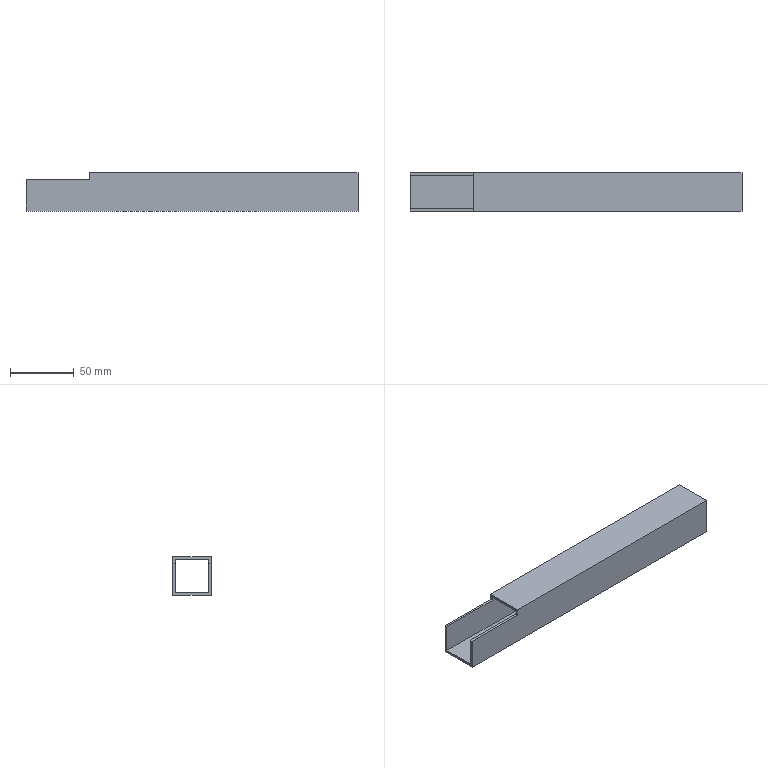Part | NX | features solid 2 | 1 solid | 13 faces | box 260 x 30 x 30 mm | volume 54640 mm3 | plane 13
STEP:
#1=CARTESIAN_POINT('',(-380.,-640.,-60.));
#2=VERTEX_POINT('',#1);
#3=CARTESIAN_POINT('',(-380.,-610.,-60.));
#4=VERTEX_POINT('',#3);
#5=CARTESIAN_POINT('',(-380.,-640.,-60.));
#6=DIRECTION('',(0.,1.,0.));
#7=VECTOR('',#6,1000.);
#8=LINE('',#5,#7);
#9=EDGE_CURVE('',#2,#4,#8,.T.);
#10=ORIENTED_EDGE('',*,*,#9,.T.);
#11=CARTESIAN_POINT('',(-380.,-610.,-30.));
#12=VERTEX_POINT('',#11);
#13=CARTESIAN_POINT('',(-380.,-610.,-30.));
#14=DIRECTION('',(0.,0.,-1.));
#15=VECTOR('',#14,1000.);
#16=LINE('',#13,#15);
#17=EDGE_CURVE('',#12,#4,#16,.T.);
#18=ORIENTED_EDGE('',*,*,#17,.F.);
#19=CARTESIAN_POINT('',(-380.,-640.,-30.));
#20=VERTEX_POINT('',#19);
#21=CARTESIAN_POINT('',(-380.,-640.,-30.));
#22=DIRECTION('',(0.,1.,0.));
#23=VECTOR('',#22,1000.);
#24=LINE('',#21,#23);
#25=EDGE_CURVE('',#20,#12,#24,.T.);
#26=ORIENTED_EDGE('',*,*,#25,.F.);
#27=CARTESIAN_POINT('',(-380.,-640.,-30.));
#28=DIRECTION('',(0.,0.,-1.));
#29=VECTOR('',#28,1000.);
#30=LINE('',#27,#29);
#31=EDGE_CURVE('',#20,#2,#30,.T.);
#32=ORIENTED_EDGE('',*,*,#31,.T.);
#33=EDGE_LOOP('',(#10,#18,#26,#32));
#34=FACE_BOUND('',#33,.T.);
#35=CARTESIAN_POINT('',(-380.,-638.,-58.));
#36=VERTEX_POINT('',#35);
#37=CARTESIAN_POINT('',(-380.,-612.,-58.));
#38=VERTEX_POINT('',#37);
#39=CARTESIAN_POINT('',(-380.,-640.,-58.));
#40=DIRECTION('',(0.,1.,0.));
#41=VECTOR('',#40,1000.);
#42=LINE('',#39,#41);
#43=EDGE_CURVE('',#36,#38,#42,.T.);
#44=ORIENTED_EDGE('',*,*,#43,.F.);
#45=CARTESIAN_POINT('',(-380.,-638.,-32.));
#46=VERTEX_POINT('',#45);
#47=CARTESIAN_POINT('',(-380.,-638.,-30.));
#48=DIRECTION('',(0.,0.,-1.));
#49=VECTOR('',#48,1000.);
#50=LINE('',#47,#49);
#51=EDGE_CURVE('',#46,#36,#50,.T.);
#52=ORIENTED_EDGE('',*,*,#51,.F.);
#53=CARTESIAN_POINT('',(-380.,-612.,-32.));
#54=VERTEX_POINT('',#53);
#55=CARTESIAN_POINT('',(-380.,-640.,-32.));
#56=DIRECTION('',(0.,1.,0.));
#57=VECTOR('',#56,1000.);
#58=LINE('',#55,#57);
#59=EDGE_CURVE('',#46,#54,#58,.T.);
#60=ORIENTED_EDGE('',*,*,#59,.T.);
#61=CARTESIAN_POINT('',(-380.,-612.,-30.));
#62=DIRECTION('',(0.,0.,-1.));
#63=VECTOR('',#62,1000.);
#64=LINE('',#61,#63);
#65=EDGE_CURVE('',#54,#38,#64,.T.);
#66=ORIENTED_EDGE('',*,*,#65,.T.);
#67=EDGE_LOOP('',(#44,#52,#60,#66));
#68=FACE_BOUND('',#67,.T.);
#69=CARTESIAN_POINT('',(-380.,-640.,-30.));
#70=DIRECTION('',(-1.,0.,0.));
#71=DIRECTION('',(0.,0.,1.));
#72=AXIS2_PLACEMENT_3D('',#69,#70,#71);
#73=PLANE('',#72);
#74=ADVANCED_FACE('',(#34,#68),#73,.F.);
#75=CARTESIAN_POINT('',(-640.,-612.,-35.));
#76=VERTEX_POINT('',#75);
#77=CARTESIAN_POINT('',(-640.,-610.,-35.));
#78=VERTEX_POINT('',#77);
#79=CARTESIAN_POINT('',(-640.,-660.,-35.));
#80=DIRECTION('',(0.,1.,0.));
#81=VECTOR('',#80,1000.);
#82=LINE('',#79,#81);
#83=EDGE_CURVE('',#76,#78,#82,.T.);
#84=ORIENTED_EDGE('',*,*,#83,.T.);
#85=CARTESIAN_POINT('',(-640.,-610.,-60.));
#86=VERTEX_POINT('',#85);
#87=CARTESIAN_POINT('',(-640.,-610.,-30.));
#88=DIRECTION('',(0.,0.,-1.));
#89=VECTOR('',#88,1000.);
#90=LINE('',#87,#89);
#91=EDGE_CURVE('',#78,#86,#90,.T.);
#92=ORIENTED_EDGE('',*,*,#91,.T.);
#93=CARTESIAN_POINT('',(-640.,-640.,-60.));
#94=VERTEX_POINT('',#93);
#95=CARTESIAN_POINT('',(-640.,-640.,-60.));
#96=DIRECTION('',(0.,1.,0.));
#97=VECTOR('',#96,1000.);
#98=LINE('',#95,#97);
#99=EDGE_CURVE('',#94,#86,#98,.T.);
#100=ORIENTED_EDGE('',*,*,#99,.F.);
#101=CARTESIAN_POINT('',(-640.,-640.,-35.));
#102=VERTEX_POINT('',#101);
#103=CARTESIAN_POINT('',(-640.,-640.,-30.));
#104=DIRECTION('',(0.,0.,-1.));
#105=VECTOR('',#104,1000.);
#106=LINE('',#103,#105);
#107=EDGE_CURVE('',#102,#94,#106,.T.);
#108=ORIENTED_EDGE('',*,*,#107,.F.);
#109=CARTESIAN_POINT('',(-640.,-638.,-35.));
#110=VERTEX_POINT('',#109);
#111=CARTESIAN_POINT('',(-640.,-660.,-35.));
#112=DIRECTION('',(0.,1.,0.));
#113=VECTOR('',#112,1000.);
#114=LINE('',#111,#113);
#115=EDGE_CURVE('',#102,#110,#114,.T.);
#116=ORIENTED_EDGE('',*,*,#115,.T.);
#117=CARTESIAN_POINT('',(-640.,-638.,-58.));
#118=VERTEX_POINT('',#117);
#119=CARTESIAN_POINT('',(-640.,-638.,-30.));
#120=DIRECTION('',(0.,0.,-1.));
#121=VECTOR('',#120,1000.);
#122=LINE('',#119,#121);
#123=EDGE_CURVE('',#110,#118,#122,.T.);
#124=ORIENTED_EDGE('',*,*,#123,.T.);
#125=CARTESIAN_POINT('',(-640.,-612.,-58.));
#126=VERTEX_POINT('',#125);
#127=CARTESIAN_POINT('',(-640.,-640.,-58.));
#128=DIRECTION('',(0.,1.,0.));
#129=VECTOR('',#128,1000.);
#130=LINE('',#127,#129);
#131=EDGE_CURVE('',#118,#126,#130,.T.);
#132=ORIENTED_EDGE('',*,*,#131,.T.);
#133=CARTESIAN_POINT('',(-640.,-612.,-30.));
#134=DIRECTION('',(0.,0.,-1.));
#135=VECTOR('',#134,1000.);
#136=LINE('',#133,#135);
#137=EDGE_CURVE('',#76,#126,#136,.T.);
#138=ORIENTED_EDGE('',*,*,#137,.F.);
#139=EDGE_LOOP('',(#84,#92,#100,#108,#116,#124,#132,#138));
#140=FACE_BOUND('',#139,.T.);
#141=CARTESIAN_POINT('',(-640.,-640.,-30.));
#142=DIRECTION('',(-1.,0.,0.));
#143=DIRECTION('',(0.,0.,1.));
#144=AXIS2_PLACEMENT_3D('',#141,#142,#143);
#145=PLANE('',#144);
#146=ADVANCED_FACE('',(#140),#145,.T.);
#147=CARTESIAN_POINT('',(-590.,-640.,-30.));
#148=VERTEX_POINT('',#147);
#149=CARTESIAN_POINT('',(-640.,-640.,-30.));
#150=DIRECTION('',(1.,0.,0.));
#151=VECTOR('',#150,1000.);
#152=LINE('',#149,#151);
#153=EDGE_CURVE('',#148,#20,#152,.T.);
#154=ORIENTED_EDGE('',*,*,#153,.F.);
#155=CARTESIAN_POINT('',(-590.,-640.,-35.));
#156=VERTEX_POINT('',#155);
#157=CARTESIAN_POINT('',(-590.,-640.,-30.));
#158=DIRECTION('',(0.,0.,-1.));
#159=VECTOR('',#158,1000.);
#160=LINE('',#157,#159);
#161=EDGE_CURVE('',#148,#156,#160,.T.);
#162=ORIENTED_EDGE('',*,*,#161,.T.);
#163=CARTESIAN_POINT('',(-640.,-640.,-35.));
#164=DIRECTION('',(-1.,0.,0.));
#165=VECTOR('',#164,1000.);
#166=LINE('',#163,#165);
#167=EDGE_CURVE('',#156,#102,#166,.T.);
#168=ORIENTED_EDGE('',*,*,#167,.T.);
#169=ORIENTED_EDGE('',*,*,#107,.T.);
#170=CARTESIAN_POINT('',(-640.,-640.,-60.));
#171=DIRECTION('',(1.,0.,0.));
#172=VECTOR('',#171,1000.);
#173=LINE('',#170,#172);
#174=EDGE_CURVE('',#94,#2,#173,.T.);
#175=ORIENTED_EDGE('',*,*,#174,.T.);
#176=ORIENTED_EDGE('',*,*,#31,.F.);
#177=EDGE_LOOP('',(#154,#162,#168,#169,#175,#176));
#178=FACE_BOUND('',#177,.T.);
#179=CARTESIAN_POINT('',(-640.,-640.,-30.));
#180=DIRECTION('',(0.,1.,0.));
#181=DIRECTION('',(0.,0.,1.));
#182=AXIS2_PLACEMENT_3D('',#179,#180,#181);
#183=PLANE('',#182);
#184=ADVANCED_FACE('',(#178),#183,.F.);
#185=CARTESIAN_POINT('',(-590.,-610.,-30.));
#186=VERTEX_POINT('',#185);
#187=CARTESIAN_POINT('',(-590.,-610.,-35.));
#188=VERTEX_POINT('',#187);
#189=CARTESIAN_POINT('',(-590.,-610.,-30.));
#190=DIRECTION('',(0.,0.,-1.));
#191=VECTOR('',#190,1000.);
#192=LINE('',#189,#191);
#193=EDGE_CURVE('',#186,#188,#192,.T.);
#194=ORIENTED_EDGE('',*,*,#193,.F.);
#195=CARTESIAN_POINT('',(-640.,-610.,-30.));
#196=DIRECTION('',(1.,0.,0.));
#197=VECTOR('',#196,1000.);
#198=LINE('',#195,#197);
#199=EDGE_CURVE('',#186,#12,#198,.T.);
#200=ORIENTED_EDGE('',*,*,#199,.T.);
#201=ORIENTED_EDGE('',*,*,#17,.T.);
#202=CARTESIAN_POINT('',(-640.,-610.,-60.));
#203=DIRECTION('',(1.,0.,0.));
#204=VECTOR('',#203,1000.);
#205=LINE('',#202,#204);
#206=EDGE_CURVE('',#86,#4,#205,.T.);
#207=ORIENTED_EDGE('',*,*,#206,.F.);
#208=ORIENTED_EDGE('',*,*,#91,.F.);
#209=CARTESIAN_POINT('',(-640.,-610.,-35.));
#210=DIRECTION('',(-1.,0.,0.));
#211=VECTOR('',#210,1000.);
#212=LINE('',#209,#211);
#213=EDGE_CURVE('',#188,#78,#212,.T.);
#214=ORIENTED_EDGE('',*,*,#213,.F.);
#215=EDGE_LOOP('',(#194,#200,#201,#207,#208,#214));
#216=FACE_BOUND('',#215,.T.);
#217=CARTESIAN_POINT('',(-640.,-610.,-30.));
#218=DIRECTION('',(0.,1.,0.));
#219=DIRECTION('',(0.,0.,1.));
#220=AXIS2_PLACEMENT_3D('',#217,#218,#219);
#221=PLANE('',#220);
#222=ADVANCED_FACE('',(#216),#221,.T.);
#223=CARTESIAN_POINT('',(-590.,-625.,-30.));
#224=DIRECTION('',(0.,1.,0.));
#225=VECTOR('',#224,1000.);
#226=LINE('',#223,#225);
#227=EDGE_CURVE('',#148,#186,#226,.T.);
#228=ORIENTED_EDGE('',*,*,#227,.F.);
#229=ORIENTED_EDGE('',*,*,#153,.T.);
#230=ORIENTED_EDGE('',*,*,#25,.T.);
#231=ORIENTED_EDGE('',*,*,#199,.F.);
#232=EDGE_LOOP('',(#228,#229,#230,#231));
#233=FACE_BOUND('',#232,.T.);
#234=CARTESIAN_POINT('',(-495.,-625.,-30.));
#235=DIRECTION('',(0.,0.,1.));
#236=DIRECTION('',(1.,0.,0.));
#237=AXIS2_PLACEMENT_3D('',#234,#235,#236);
#238=PLANE('',#237);
#239=ADVANCED_FACE('',(#233),#238,.T.);
#240=ORIENTED_EDGE('',*,*,#174,.F.);
#241=ORIENTED_EDGE('',*,*,#99,.T.);
#242=ORIENTED_EDGE('',*,*,#206,.T.);
#243=ORIENTED_EDGE('',*,*,#9,.F.);
#244=EDGE_LOOP('',(#240,#241,#242,#243));
#245=FACE_BOUND('',#244,.T.);
#246=CARTESIAN_POINT('',(-495.,-625.,-60.));
#247=DIRECTION('',(0.,0.,1.));
#248=DIRECTION('',(1.,0.,0.));
#249=AXIS2_PLACEMENT_3D('',#246,#247,#248);
#250=PLANE('',#249);
#251=ADVANCED_FACE('',(#245),#250,.F.);
#252=CARTESIAN_POINT('',(-590.,-638.,-32.));
#253=VERTEX_POINT('',#252);
#254=CARTESIAN_POINT('',(-590.,-638.,-35.));
#255=VERTEX_POINT('',#254);
#256=CARTESIAN_POINT('',(-590.,-638.,-30.));
#257=DIRECTION('',(0.,0.,-1.));
#258=VECTOR('',#257,1000.);
#259=LINE('',#256,#258);
#260=EDGE_CURVE('',#253,#255,#259,.T.);
#261=ORIENTED_EDGE('',*,*,#260,.F.);
#262=CARTESIAN_POINT('',(-640.,-638.,-32.));
#263=DIRECTION('',(1.,0.,0.));
#264=VECTOR('',#263,1000.);
#265=LINE('',#262,#264);
#266=EDGE_CURVE('',#253,#46,#265,.T.);
#267=ORIENTED_EDGE('',*,*,#266,.T.);
#268=ORIENTED_EDGE('',*,*,#51,.T.);
#269=CARTESIAN_POINT('',(-640.,-638.,-58.));
#270=DIRECTION('',(1.,0.,0.));
#271=VECTOR('',#270,1000.);
#272=LINE('',#269,#271);
#273=EDGE_CURVE('',#118,#36,#272,.T.);
#274=ORIENTED_EDGE('',*,*,#273,.F.);
#275=ORIENTED_EDGE('',*,*,#123,.F.);
#276=CARTESIAN_POINT('',(-640.,-638.,-35.));
#277=DIRECTION('',(-1.,0.,0.));
#278=VECTOR('',#277,1000.);
#279=LINE('',#276,#278);
#280=EDGE_CURVE('',#255,#110,#279,.T.);
#281=ORIENTED_EDGE('',*,*,#280,.F.);
#282=EDGE_LOOP('',(#261,#267,#268,#274,#275,#281));
#283=FACE_BOUND('',#282,.T.);
#284=CARTESIAN_POINT('',(-640.,-638.,-30.));
#285=DIRECTION('',(0.,1.,0.));
#286=DIRECTION('',(0.,0.,1.));
#287=AXIS2_PLACEMENT_3D('',#284,#285,#286);
#288=PLANE('',#287);
#289=ADVANCED_FACE('',(#283),#288,.T.);
#290=CARTESIAN_POINT('',(-590.,-612.,-32.));
#291=VERTEX_POINT('',#290);
#292=CARTESIAN_POINT('',(-640.,-612.,-32.));
#293=DIRECTION('',(1.,0.,0.));
#294=VECTOR('',#293,1000.);
#295=LINE('',#292,#294);
#296=EDGE_CURVE('',#291,#54,#295,.T.);
#297=ORIENTED_EDGE('',*,*,#296,.F.);
#298=CARTESIAN_POINT('',(-590.,-612.,-35.));
#299=VERTEX_POINT('',#298);
#300=CARTESIAN_POINT('',(-590.,-612.,-30.));
#301=DIRECTION('',(0.,0.,-1.));
#302=VECTOR('',#301,1000.);
#303=LINE('',#300,#302);
#304=EDGE_CURVE('',#291,#299,#303,.T.);
#305=ORIENTED_EDGE('',*,*,#304,.T.);
#306=CARTESIAN_POINT('',(-640.,-612.,-35.));
#307=DIRECTION('',(-1.,0.,0.));
#308=VECTOR('',#307,1000.);
#309=LINE('',#306,#308);
#310=EDGE_CURVE('',#299,#76,#309,.T.);
#311=ORIENTED_EDGE('',*,*,#310,.T.);
#312=ORIENTED_EDGE('',*,*,#137,.T.);
#313=CARTESIAN_POINT('',(-640.,-612.,-58.));
#314=DIRECTION('',(1.,0.,0.));
#315=VECTOR('',#314,1000.);
#316=LINE('',#313,#315);
#317=EDGE_CURVE('',#126,#38,#316,.T.);
#318=ORIENTED_EDGE('',*,*,#317,.T.);
#319=ORIENTED_EDGE('',*,*,#65,.F.);
#320=EDGE_LOOP('',(#297,#305,#311,#312,#318,#319));
#321=FACE_BOUND('',#320,.T.);
#322=CARTESIAN_POINT('',(-640.,-612.,-30.));
#323=DIRECTION('',(0.,1.,0.));
#324=DIRECTION('',(0.,0.,1.));
#325=AXIS2_PLACEMENT_3D('',#322,#323,#324);
#326=PLANE('',#325);
#327=ADVANCED_FACE('',(#321),#326,.F.);
#328=ORIENTED_EDGE('',*,*,#266,.F.);
#329=CARTESIAN_POINT('',(-590.,-625.,-32.));
#330=DIRECTION('',(0.,1.,0.));
#331=VECTOR('',#330,1000.);
#332=LINE('',#329,#331);
#333=EDGE_CURVE('',#253,#291,#332,.T.);
#334=ORIENTED_EDGE('',*,*,#333,.T.);
#335=ORIENTED_EDGE('',*,*,#296,.T.);
#336=ORIENTED_EDGE('',*,*,#59,.F.);
#337=EDGE_LOOP('',(#328,#334,#335,#336));
#338=FACE_BOUND('',#337,.T.);
#339=CARTESIAN_POINT('',(-495.,-625.,-32.));
#340=DIRECTION('',(0.,0.,1.));
#341=DIRECTION('',(1.,0.,0.));
#342=AXIS2_PLACEMENT_3D('',#339,#340,#341);
#343=PLANE('',#342);
#344=ADVANCED_FACE('',(#338),#343,.F.);
#345=ORIENTED_EDGE('',*,*,#273,.T.);
#346=ORIENTED_EDGE('',*,*,#43,.T.);
#347=ORIENTED_EDGE('',*,*,#317,.F.);
#348=ORIENTED_EDGE('',*,*,#131,.F.);
#349=EDGE_LOOP('',(#345,#346,#347,#348));
#350=FACE_BOUND('',#349,.T.);
#351=CARTESIAN_POINT('',(-495.,-625.,-58.));
#352=DIRECTION('',(0.,0.,1.));
#353=DIRECTION('',(1.,0.,0.));
#354=AXIS2_PLACEMENT_3D('',#351,#352,#353);
#355=PLANE('',#354);
#356=ADVANCED_FACE('',(#350),#355,.T.);
#357=CARTESIAN_POINT('',(-590.,-660.,-35.));
#358=DIRECTION('',(0.,1.,0.));
#359=VECTOR('',#358,1000.);
#360=LINE('',#357,#359);
#361=EDGE_CURVE('',#156,#255,#360,.T.);
#362=ORIENTED_EDGE('',*,*,#361,.T.);
#363=ORIENTED_EDGE('',*,*,#280,.T.);
#364=ORIENTED_EDGE('',*,*,#115,.F.);
#365=ORIENTED_EDGE('',*,*,#167,.F.);
#366=EDGE_LOOP('',(#362,#363,#364,#365));
#367=FACE_BOUND('',#366,.T.);
#368=CARTESIAN_POINT('',(-590.,-660.,-35.));
#369=DIRECTION('',(0.,0.,-1.));
#370=DIRECTION('',(0.,-1.,0.));
#371=AXIS2_PLACEMENT_3D('',#368,#369,#370);
#372=PLANE('',#371);
#373=ADVANCED_FACE('',(#367),#372,.F.);
#374=ORIENTED_EDGE('',*,*,#213,.T.);
#375=ORIENTED_EDGE('',*,*,#83,.F.);
#376=ORIENTED_EDGE('',*,*,#310,.F.);
#377=CARTESIAN_POINT('',(-590.,-660.,-35.));
#378=DIRECTION('',(0.,1.,0.));
#379=VECTOR('',#378,1000.);
#380=LINE('',#377,#379);
#381=EDGE_CURVE('',#299,#188,#380,.T.);
#382=ORIENTED_EDGE('',*,*,#381,.T.);
#383=EDGE_LOOP('',(#374,#375,#376,#382));
#384=FACE_BOUND('',#383,.T.);
#385=CARTESIAN_POINT('',(-590.,-660.,-35.));
#386=DIRECTION('',(0.,0.,-1.));
#387=DIRECTION('',(0.,-1.,0.));
#388=AXIS2_PLACEMENT_3D('',#385,#386,#387);
#389=PLANE('',#388);
#390=ADVANCED_FACE('',(#384),#389,.F.);
#391=ORIENTED_EDGE('',*,*,#227,.T.);
#392=ORIENTED_EDGE('',*,*,#193,.T.);
#393=ORIENTED_EDGE('',*,*,#381,.F.);
#394=ORIENTED_EDGE('',*,*,#304,.F.);
#395=ORIENTED_EDGE('',*,*,#333,.F.);
#396=ORIENTED_EDGE('',*,*,#260,.T.);
#397=ORIENTED_EDGE('',*,*,#361,.F.);
#398=ORIENTED_EDGE('',*,*,#161,.F.);
#399=EDGE_LOOP('',(#391,#392,#393,#394,#395,#396,#397,#398));
#400=FACE_BOUND('',#399,.T.);
#401=CARTESIAN_POINT('',(-590.,-660.,-3.));
#402=DIRECTION('',(1.,0.,0.));
#403=DIRECTION('',(0.,0.,-1.));
#404=AXIS2_PLACEMENT_3D('',#401,#402,#403);
#405=PLANE('',#404);
#406=ADVANCED_FACE('',(#400),#405,.F.);
#407=CLOSED_SHELL('',(#74,#146,#184,#222,#239,#251,#289,#327,#344,#356,#373,#390,#406));
#408=MANIFOLD_SOLID_BREP('',#407);
#409=(LENGTH_UNIT()NAMED_UNIT(*)SI_UNIT(.MILLI.,.METRE.));
#410=UNCERTAINTY_MEASURE_WITH_UNIT(LENGTH_MEASURE(0.00001),#409,'','');
#411=(NAMED_UNIT(*)PLANE_ANGLE_UNIT()SI_UNIT($,.RADIAN.));
#412=(NAMED_UNIT(*)SI_UNIT($,.STERADIAN.)SOLID_ANGLE_UNIT());
#413=(GEOMETRIC_REPRESENTATION_CONTEXT(3)GLOBAL_UNCERTAINTY_ASSIGNED_CONTEXT((#410))GLOBAL_UNIT_ASSIGNED_CONTEXT((#409,#411,#412))REPRESENTATION_CONTEXT('',''));
#414=ADVANCED_BREP_SHAPE_REPRESENTATION('',(#408),#413);